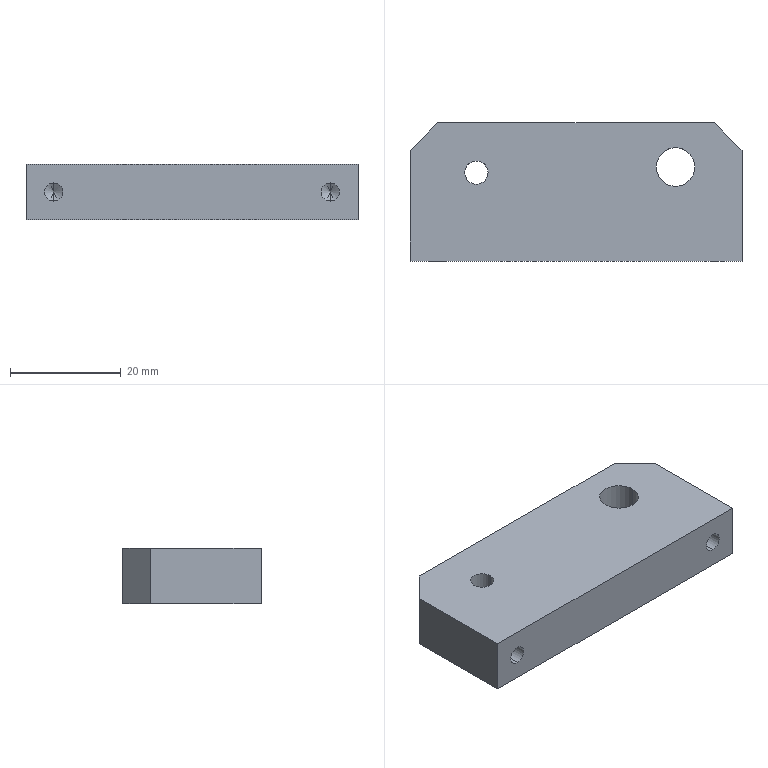Part | STEP file | 2077 Cylinder mounting plate | 1 solid | 20 faces | box 60 x 25 x 10 mm | volume 14024 mm3 | cylinder 8 | plane 8 | cone 4 | commonest cylinder face diameters 3.3 x4 4.2 x2 7 x2
STEP:
#1=CARTESIAN_POINT('',(0.,0.,0.));
#2=DIRECTION('',(0.,0.,1.));
#3=DIRECTION('',(1.,0.,0.));
#4=AXIS2_PLACEMENT_3D('',#1,#2,#3);
#5=CARTESIAN_POINT('',(-15.9,3.5,0.));
#6=VERTEX_POINT('',#5);
#7=CARTESIAN_POINT('',(-15.9,3.5,10.));
#8=VERTEX_POINT('',#7);
#9=CARTESIAN_POINT('',(-15.9,3.5,10.));
#10=DIRECTION('',(0.,0.,1.));
#11=VECTOR('',#10,1.);
#12=LINE('',#9,#11);
#13=CARTESIAN_POINT('',(-18.,3.5,10.));
#14=DIRECTION('',(0.,0.,1.));
#15=DIRECTION('',(1.,0.,0.));
#16=AXIS2_PLACEMENT_3D('',#13,#14,#15);
#17=CYLINDRICAL_SURFACE('',#16,2.1);
#18=CARTESIAN_POINT('',(6.283,0.));
#19=DIRECTION('',(0.,1.));
#20=VECTOR('',#19,1.);
#21=LINE('',#18,#20);
#22=(GEOMETRIC_REPRESENTATION_CONTEXT(2)PARAMETRIC_REPRESENTATION_CONTEXT()REPRESENTATION_CONTEXT('',''));
#23=DEFINITIONAL_REPRESENTATION('',(#21),#22);
#24=PCURVE('',#17,#23);
#25=CARTESIAN_POINT('',(-18.,3.5,10.));
#26=DIRECTION('',(0.,0.,1.));
#27=DIRECTION('',(1.,0.,0.));
#28=AXIS2_PLACEMENT_3D('',#25,#26,#27);
#29=CYLINDRICAL_SURFACE('',#28,2.1);
#30=CARTESIAN_POINT('',(0.,0.));
#31=DIRECTION('',(0.,1.));
#32=VECTOR('',#31,1.);
#33=LINE('',#30,#32);
#34=(GEOMETRIC_REPRESENTATION_CONTEXT(2)PARAMETRIC_REPRESENTATION_CONTEXT()REPRESENTATION_CONTEXT('',''));
#35=DEFINITIONAL_REPRESENTATION('',(#33),#34);
#36=PCURVE('',#29,#35);
#37=SURFACE_CURVE('',#12,(#24,#36),.PCURVE_S1.);
#38=EDGE_CURVE('',#6,#8,#37,.T.);
#39=ORIENTED_EDGE('',*,*,#38,.T.);
#40=CARTESIAN_POINT('',(-20.1,3.5,10.));
#41=VERTEX_POINT('',#40);
#42=CARTESIAN_POINT('',(-18.,3.5,10.));
#43=DIRECTION('',(0.,0.,1.));
#44=DIRECTION('',(1.,0.,0.));
#45=AXIS2_PLACEMENT_3D('',#42,#43,#44);
#46=CIRCLE('',#45,2.1);
#47=CARTESIAN_POINT('',(0.,0.));
#48=DIRECTION('',(1.,0.));
#49=VECTOR('',#48,1.);
#50=LINE('',#47,#49);
#51=(GEOMETRIC_REPRESENTATION_CONTEXT(2)PARAMETRIC_REPRESENTATION_CONTEXT()REPRESENTATION_CONTEXT('',''));
#52=DEFINITIONAL_REPRESENTATION('',(#50),#51);
#53=PCURVE('',#17,#52);
#54=CARTESIAN_POINT('',(0.,0.,10.));
#55=DIRECTION('',(0.,0.,-1.));
#56=DIRECTION('',(-1.,0.,0.));
#57=AXIS2_PLACEMENT_3D('',#54,#55,#56);
#58=PLANE('',#57);
#59=CARTESIAN_POINT('',(15.9,3.5));
#60=CARTESIAN_POINT('',(15.9,7.137));
#61=CARTESIAN_POINT('',(19.05,5.319));
#62=CARTESIAN_POINT('',(22.2,3.5));
#63=CARTESIAN_POINT('',(19.05,1.681));
#64=CARTESIAN_POINT('',(15.9,-0.1373));
#65=CARTESIAN_POINT('',(15.9,3.5));
#66=(BOUNDED_CURVE()B_SPLINE_CURVE(2,(#59,#60,#61,#62,#63,#64,#65),.UNSPECIFIED.,.T.,.F.)B_SPLINE_CURVE_WITH_KNOTS((1,2,2,2,2,1),(-2.094,0.,2.094,4.189,6.283,8.378),.UNSPECIFIED.)CURVE()GEOMETRIC_REPRESENTATION_ITEM()RATIONAL_B_SPLINE_CURVE((1.,0.5,1.,0.5,1.,0.5,1.))REPRESENTATION_ITEM(''));
#67=(GEOMETRIC_REPRESENTATION_CONTEXT(2)PARAMETRIC_REPRESENTATION_CONTEXT()REPRESENTATION_CONTEXT('',''));
#68=DEFINITIONAL_REPRESENTATION('',(#66),#67);
#69=PCURVE('',#58,#68);
#70=SURFACE_CURVE('',#46,(#53,#69),.PCURVE_S1.);
#71=EDGE_CURVE('',#41,#8,#70,.T.);
#72=ORIENTED_EDGE('',*,*,#71,.F.);
#73=CARTESIAN_POINT('',(-20.1,3.5,0.));
#74=VERTEX_POINT('',#73);
#75=CARTESIAN_POINT('',(-20.1,3.5,10.));
#76=DIRECTION('',(0.,0.,1.));
#77=VECTOR('',#76,1.);
#78=LINE('',#75,#77);
#79=CARTESIAN_POINT('',(3.142,0.));
#80=DIRECTION('',(0.,1.));
#81=VECTOR('',#80,1.);
#82=LINE('',#79,#81);
#83=(GEOMETRIC_REPRESENTATION_CONTEXT(2)PARAMETRIC_REPRESENTATION_CONTEXT()REPRESENTATION_CONTEXT('',''));
#84=DEFINITIONAL_REPRESENTATION('',(#82),#83);
#85=PCURVE('',#17,#84);
#86=CARTESIAN_POINT('',(3.142,0.));
#87=DIRECTION('',(0.,1.));
#88=VECTOR('',#87,1.);
#89=LINE('',#86,#88);
#90=(GEOMETRIC_REPRESENTATION_CONTEXT(2)PARAMETRIC_REPRESENTATION_CONTEXT()REPRESENTATION_CONTEXT('',''));
#91=DEFINITIONAL_REPRESENTATION('',(#89),#90);
#92=PCURVE('',#29,#91);
#93=SURFACE_CURVE('',#78,(#85,#92),.PCURVE_S1.);
#94=EDGE_CURVE('',#74,#41,#93,.T.);
#95=ORIENTED_EDGE('',*,*,#94,.F.);
#96=CARTESIAN_POINT('',(-18.,3.5,0.));
#97=DIRECTION('',(0.,0.,1.));
#98=DIRECTION('',(1.,0.,0.));
#99=AXIS2_PLACEMENT_3D('',#96,#97,#98);
#100=CIRCLE('',#99,2.1);
#101=CARTESIAN_POINT('',(0.,-10.));
#102=DIRECTION('',(1.,0.));
#103=VECTOR('',#102,1.);
#104=LINE('',#101,#103);
#105=(GEOMETRIC_REPRESENTATION_CONTEXT(2)PARAMETRIC_REPRESENTATION_CONTEXT()REPRESENTATION_CONTEXT('',''));
#106=DEFINITIONAL_REPRESENTATION('',(#104),#105);
#107=PCURVE('',#17,#106);
#108=CARTESIAN_POINT('',(0.,0.,0.));
#109=DIRECTION('',(0.,0.,-1.));
#110=DIRECTION('',(-1.,0.,0.));
#111=AXIS2_PLACEMENT_3D('',#108,#109,#110);
#112=PLANE('',#111);
#113=CARTESIAN_POINT('',(15.9,3.5));
#114=CARTESIAN_POINT('',(15.9,7.137));
#115=CARTESIAN_POINT('',(19.05,5.319));
#116=CARTESIAN_POINT('',(22.2,3.5));
#117=CARTESIAN_POINT('',(19.05,1.681));
#118=CARTESIAN_POINT('',(15.9,-0.1373));
#119=CARTESIAN_POINT('',(15.9,3.5));
#120=(BOUNDED_CURVE()B_SPLINE_CURVE(2,(#113,#114,#115,#116,#117,#118,#119),.UNSPECIFIED.,.T.,.F.)B_SPLINE_CURVE_WITH_KNOTS((1,2,2,2,2,1),(-2.094,0.,2.094,4.189,6.283,8.378),.UNSPECIFIED.)CURVE()GEOMETRIC_REPRESENTATION_ITEM()RATIONAL_B_SPLINE_CURVE((1.,0.5,1.,0.5,1.,0.5,1.))REPRESENTATION_ITEM(''));
#121=(GEOMETRIC_REPRESENTATION_CONTEXT(2)PARAMETRIC_REPRESENTATION_CONTEXT()REPRESENTATION_CONTEXT('',''));
#122=DEFINITIONAL_REPRESENTATION('',(#120),#121);
#123=PCURVE('',#112,#122);
#124=SURFACE_CURVE('',#100,(#107,#123),.PCURVE_S1.);
#125=EDGE_CURVE('',#74,#6,#124,.T.);
#126=ORIENTED_EDGE('',*,*,#125,.T.);
#127=EDGE_LOOP('',(#39,#72,#95,#126));
#128=FACE_BOUND('',#127,.F.);
#129=ADVANCED_FACE('',(#128),#17,.F.);
#130=CARTESIAN_POINT('',(21.5,4.5,0.));
#131=VERTEX_POINT('',#130);
#132=CARTESIAN_POINT('',(21.5,4.5,10.));
#133=VERTEX_POINT('',#132);
#134=CARTESIAN_POINT('',(21.5,4.5,10.));
#135=DIRECTION('',(0.,0.,1.));
#136=VECTOR('',#135,1.);
#137=LINE('',#134,#136);
#138=CARTESIAN_POINT('',(18.,4.5,10.));
#139=DIRECTION('',(0.,0.,1.));
#140=DIRECTION('',(1.,0.,0.));
#141=AXIS2_PLACEMENT_3D('',#138,#139,#140);
#142=CYLINDRICAL_SURFACE('',#141,3.5);
#143=CARTESIAN_POINT('',(6.283,0.));
#144=DIRECTION('',(0.,1.));
#145=VECTOR('',#144,1.);
#146=LINE('',#143,#145);
#147=(GEOMETRIC_REPRESENTATION_CONTEXT(2)PARAMETRIC_REPRESENTATION_CONTEXT()REPRESENTATION_CONTEXT('',''));
#148=DEFINITIONAL_REPRESENTATION('',(#146),#147);
#149=PCURVE('',#142,#148);
#150=CARTESIAN_POINT('',(18.,4.5,10.));
#151=DIRECTION('',(0.,0.,1.));
#152=DIRECTION('',(1.,0.,0.));
#153=AXIS2_PLACEMENT_3D('',#150,#151,#152);
#154=CYLINDRICAL_SURFACE('',#153,3.5);
#155=CARTESIAN_POINT('',(0.,0.));
#156=DIRECTION('',(0.,1.));
#157=VECTOR('',#156,1.);
#158=LINE('',#155,#157);
#159=(GEOMETRIC_REPRESENTATION_CONTEXT(2)PARAMETRIC_REPRESENTATION_CONTEXT()REPRESENTATION_CONTEXT('',''));
#160=DEFINITIONAL_REPRESENTATION('',(#158),#159);
#161=PCURVE('',#154,#160);
#162=SURFACE_CURVE('',#137,(#149,#161),.PCURVE_S1.);
#163=EDGE_CURVE('',#131,#133,#162,.T.);
#164=ORIENTED_EDGE('',*,*,#163,.T.);
#165=CARTESIAN_POINT('',(14.5,4.5,10.));
#166=VERTEX_POINT('',#165);
#167=CARTESIAN_POINT('',(18.,4.5,10.));
#168=DIRECTION('',(0.,0.,1.));
#169=DIRECTION('',(1.,0.,0.));
#170=AXIS2_PLACEMENT_3D('',#167,#168,#169);
#171=CIRCLE('',#170,3.5);
#172=CARTESIAN_POINT('',(0.,0.));
#173=DIRECTION('',(1.,0.));
#174=VECTOR('',#173,1.);
#175=LINE('',#172,#174);
#176=(GEOMETRIC_REPRESENTATION_CONTEXT(2)PARAMETRIC_REPRESENTATION_CONTEXT()REPRESENTATION_CONTEXT('',''));
#177=DEFINITIONAL_REPRESENTATION('',(#175),#176);
#178=PCURVE('',#142,#177);
#179=CARTESIAN_POINT('',(-21.5,4.5));
#180=CARTESIAN_POINT('',(-21.5,10.562));
#181=CARTESIAN_POINT('',(-16.25,7.531));
#182=CARTESIAN_POINT('',(-11.,4.5));
#183=CARTESIAN_POINT('',(-16.25,1.469));
#184=CARTESIAN_POINT('',(-21.5,-1.562));
#185=CARTESIAN_POINT('',(-21.5,4.5));
#186=(BOUNDED_CURVE()B_SPLINE_CURVE(2,(#179,#180,#181,#182,#183,#184,#185),.UNSPECIFIED.,.T.,.F.)B_SPLINE_CURVE_WITH_KNOTS((1,2,2,2,2,1),(-2.094,0.,2.094,4.189,6.283,8.378),.UNSPECIFIED.)CURVE()GEOMETRIC_REPRESENTATION_ITEM()RATIONAL_B_SPLINE_CURVE((1.,0.5,1.,0.5,1.,0.5,1.))REPRESENTATION_ITEM(''));
#187=(GEOMETRIC_REPRESENTATION_CONTEXT(2)PARAMETRIC_REPRESENTATION_CONTEXT()REPRESENTATION_CONTEXT('',''));
#188=DEFINITIONAL_REPRESENTATION('',(#186),#187);
#189=PCURVE('',#58,#188);
#190=SURFACE_CURVE('',#171,(#178,#189),.PCURVE_S1.);
#191=EDGE_CURVE('',#166,#133,#190,.T.);
#192=ORIENTED_EDGE('',*,*,#191,.F.);
#193=CARTESIAN_POINT('',(14.5,4.5,0.));
#194=VERTEX_POINT('',#193);
#195=CARTESIAN_POINT('',(14.5,4.5,10.));
#196=DIRECTION('',(0.,0.,1.));
#197=VECTOR('',#196,1.);
#198=LINE('',#195,#197);
#199=CARTESIAN_POINT('',(3.142,0.));
#200=DIRECTION('',(0.,1.));
#201=VECTOR('',#200,1.);
#202=LINE('',#199,#201);
#203=(GEOMETRIC_REPRESENTATION_CONTEXT(2)PARAMETRIC_REPRESENTATION_CONTEXT()REPRESENTATION_CONTEXT('',''));
#204=DEFINITIONAL_REPRESENTATION('',(#202),#203);
#205=PCURVE('',#142,#204);
#206=CARTESIAN_POINT('',(3.142,0.));
#207=DIRECTION('',(0.,1.));
#208=VECTOR('',#207,1.);
#209=LINE('',#206,#208);
#210=(GEOMETRIC_REPRESENTATION_CONTEXT(2)PARAMETRIC_REPRESENTATION_CONTEXT()REPRESENTATION_CONTEXT('',''));
#211=DEFINITIONAL_REPRESENTATION('',(#209),#210);
#212=PCURVE('',#154,#211);
#213=SURFACE_CURVE('',#198,(#205,#212),.PCURVE_S1.);
#214=EDGE_CURVE('',#194,#166,#213,.T.);
#215=ORIENTED_EDGE('',*,*,#214,.F.);
#216=CARTESIAN_POINT('',(18.,4.5,0.));
#217=DIRECTION('',(0.,0.,1.));
#218=DIRECTION('',(1.,0.,0.));
#219=AXIS2_PLACEMENT_3D('',#216,#217,#218);
#220=CIRCLE('',#219,3.5);
#221=CARTESIAN_POINT('',(0.,-10.));
#222=DIRECTION('',(1.,0.));
#223=VECTOR('',#222,1.);
#224=LINE('',#221,#223);
#225=(GEOMETRIC_REPRESENTATION_CONTEXT(2)PARAMETRIC_REPRESENTATION_CONTEXT()REPRESENTATION_CONTEXT('',''));
#226=DEFINITIONAL_REPRESENTATION('',(#224),#225);
#227=PCURVE('',#142,#226);
#228=CARTESIAN_POINT('',(-21.5,4.5));
#229=CARTESIAN_POINT('',(-21.5,10.562));
#230=CARTESIAN_POINT('',(-16.25,7.531));
#231=CARTESIAN_POINT('',(-11.,4.5));
#232=CARTESIAN_POINT('',(-16.25,1.469));
#233=CARTESIAN_POINT('',(-21.5,-1.562));
#234=CARTESIAN_POINT('',(-21.5,4.5));
#235=(BOUNDED_CURVE()B_SPLINE_CURVE(2,(#228,#229,#230,#231,#232,#233,#234),.UNSPECIFIED.,.T.,.F.)B_SPLINE_CURVE_WITH_KNOTS((1,2,2,2,2,1),(-2.094,0.,2.094,4.189,6.283,8.378),.UNSPECIFIED.)CURVE()GEOMETRIC_REPRESENTATION_ITEM()RATIONAL_B_SPLINE_CURVE((1.,0.5,1.,0.5,1.,0.5,1.))REPRESENTATION_ITEM(''));
#236=(GEOMETRIC_REPRESENTATION_CONTEXT(2)PARAMETRIC_REPRESENTATION_CONTEXT()REPRESENTATION_CONTEXT('',''));
#237=DEFINITIONAL_REPRESENTATION('',(#235),#236);
#238=PCURVE('',#112,#237);
#239=SURFACE_CURVE('',#220,(#227,#238),.PCURVE_S1.);
#240=EDGE_CURVE('',#194,#131,#239,.T.);
#241=ORIENTED_EDGE('',*,*,#240,.T.);
#242=EDGE_LOOP('',(#164,#192,#215,#241));
#243=FACE_BOUND('',#242,.F.);
#244=ADVANCED_FACE('',(#243),#142,.F.);
#245=CARTESIAN_POINT('',(25.,-1.,3.35));
#246=VERTEX_POINT('',#245);
#247=CARTESIAN_POINT('',(25.,-12.5,3.35));
#248=VERTEX_POINT('',#247);
#249=CARTESIAN_POINT('',(25.,-12.5,3.35));
#250=DIRECTION('',(0.,-1.,0.));
#251=VECTOR('',#250,1.);
#252=LINE('',#249,#251);
#253=CARTESIAN_POINT('',(25.,-12.5,5.));
#254=DIRECTION('',(0.,-1.,0.));
#255=DIRECTION('',(0.,0.,-1.));
#256=AXIS2_PLACEMENT_3D('',#253,#254,#255);
#257=CYLINDRICAL_SURFACE('',#256,1.65);
#258=CARTESIAN_POINT('',(6.283,0.));
#259=DIRECTION('',(0.,1.));
#260=VECTOR('',#259,1.);
#261=LINE('',#258,#260);
#262=(GEOMETRIC_REPRESENTATION_CONTEXT(2)PARAMETRIC_REPRESENTATION_CONTEXT()REPRESENTATION_CONTEXT('',''));
#263=DEFINITIONAL_REPRESENTATION('',(#261),#262);
#264=PCURVE('',#257,#263);
#265=CARTESIAN_POINT('',(25.,-12.5,5.));
#266=DIRECTION('',(0.,-1.,0.));
#267=DIRECTION('',(0.,0.,-1.));
#268=AXIS2_PLACEMENT_3D('',#265,#266,#267);
#269=CYLINDRICAL_SURFACE('',#268,1.65);
#270=CARTESIAN_POINT('',(0.,0.));
#271=DIRECTION('',(0.,1.));
#272=VECTOR('',#271,1.);
#273=LINE('',#270,#272);
#274=(GEOMETRIC_REPRESENTATION_CONTEXT(2)PARAMETRIC_REPRESENTATION_CONTEXT()REPRESENTATION_CONTEXT('',''));
#275=DEFINITIONAL_REPRESENTATION('',(#273),#274);
#276=PCURVE('',#269,#275);
#277=SURFACE_CURVE('',#252,(#264,#276),.PCURVE_S1.);
#278=EDGE_CURVE('',#246,#248,#277,.T.);
#279=ORIENTED_EDGE('',*,*,#278,.T.);
#280=CARTESIAN_POINT('',(25.,-12.5,6.65));
#281=VERTEX_POINT('',#280);
#282=CARTESIAN_POINT('',(25.,-12.5,5.));
#283=DIRECTION('',(0.,-1.,0.));
#284=DIRECTION('',(0.,0.,-1.));
#285=AXIS2_PLACEMENT_3D('',#282,#283,#284);
#286=CIRCLE('',#285,1.65);
#287=CARTESIAN_POINT('',(0.,0.));
#288=DIRECTION('',(1.,0.));
#289=VECTOR('',#288,1.);
#290=LINE('',#287,#289);
#291=(GEOMETRIC_REPRESENTATION_CONTEXT(2)PARAMETRIC_REPRESENTATION_CONTEXT()REPRESENTATION_CONTEXT('',''));
#292=DEFINITIONAL_REPRESENTATION('',(#290),#291);
#293=PCURVE('',#257,#292);
#294=CARTESIAN_POINT('',(-30.,-12.5,10.));
#295=DIRECTION('',(0.,1.,0.));
#296=DIRECTION('',(0.,0.,1.));
#297=AXIS2_PLACEMENT_3D('',#294,#295,#296);
#298=PLANE('',#297);
#299=CARTESIAN_POINT('',(-6.65,55.));
#300=CARTESIAN_POINT('',(-6.65,57.858));
#301=CARTESIAN_POINT('',(-4.175,56.429));
#302=CARTESIAN_POINT('',(-1.7,55.));
#303=CARTESIAN_POINT('',(-4.175,53.571));
#304=CARTESIAN_POINT('',(-6.65,52.142));
#305=CARTESIAN_POINT('',(-6.65,55.));
#306=(BOUNDED_CURVE()B_SPLINE_CURVE(2,(#299,#300,#301,#302,#303,#304,#305),.UNSPECIFIED.,.T.,.F.)B_SPLINE_CURVE_WITH_KNOTS((1,2,2,2,2,1),(-2.094,0.,2.094,4.189,6.283,8.378),.UNSPECIFIED.)CURVE()GEOMETRIC_REPRESENTATION_ITEM()RATIONAL_B_SPLINE_CURVE((1.,0.5,1.,0.5,1.,0.5,1.))REPRESENTATION_ITEM(''));
#307=(GEOMETRIC_REPRESENTATION_CONTEXT(2)PARAMETRIC_REPRESENTATION_CONTEXT()REPRESENTATION_CONTEXT('',''));
#308=DEFINITIONAL_REPRESENTATION('',(#306),#307);
#309=PCURVE('',#298,#308);
#310=SURFACE_CURVE('',#286,(#293,#309),.PCURVE_S1.);
#311=EDGE_CURVE('',#281,#248,#310,.T.);
#312=ORIENTED_EDGE('',*,*,#311,.F.);
#313=CARTESIAN_POINT('',(25.,-1.,6.65));
#314=VERTEX_POINT('',#313);
#315=CARTESIAN_POINT('',(25.,-12.5,6.65));
#316=DIRECTION('',(0.,-1.,0.));
#317=VECTOR('',#316,1.);
#318=LINE('',#315,#317);
#319=CARTESIAN_POINT('',(3.142,0.));
#320=DIRECTION('',(0.,1.));
#321=VECTOR('',#320,1.);
#322=LINE('',#319,#321);
#323=(GEOMETRIC_REPRESENTATION_CONTEXT(2)PARAMETRIC_REPRESENTATION_CONTEXT()REPRESENTATION_CONTEXT('',''));
#324=DEFINITIONAL_REPRESENTATION('',(#322),#323);
#325=PCURVE('',#257,#324);
#326=CARTESIAN_POINT('',(3.142,0.));
#327=DIRECTION('',(0.,1.));
#328=VECTOR('',#327,1.);
#329=LINE('',#326,#328);
#330=(GEOMETRIC_REPRESENTATION_CONTEXT(2)PARAMETRIC_REPRESENTATION_CONTEXT()REPRESENTATION_CONTEXT('',''));
#331=DEFINITIONAL_REPRESENTATION('',(#329),#330);
#332=PCURVE('',#269,#331);
#333=SURFACE_CURVE('',#318,(#325,#332),.PCURVE_S1.);
#334=EDGE_CURVE('',#314,#281,#333,.T.);
#335=ORIENTED_EDGE('',*,*,#334,.F.);
#336=CARTESIAN_POINT('',(25.,-1.,5.));
#337=DIRECTION('',(0.,-1.,0.));
#338=DIRECTION('',(0.,0.,-1.));
#339=AXIS2_PLACEMENT_3D('',#336,#337,#338);
#340=CIRCLE('',#339,1.65);
#341=CARTESIAN_POINT('',(0.,-11.5));
#342=DIRECTION('',(1.,0.));
#343=VECTOR('',#342,1.);
#344=LINE('',#341,#343);
#345=(GEOMETRIC_REPRESENTATION_CONTEXT(2)PARAMETRIC_REPRESENTATION_CONTEXT()REPRESENTATION_CONTEXT('',''));
#346=DEFINITIONAL_REPRESENTATION('',(#344),#345);
#347=PCURVE('',#257,#346);
#348=CARTESIAN_POINT('',(25.,-1.,5.));
#349=DIRECTION('',(0.,-1.,0.));
#350=DIRECTION('',(0.,0.,-1.));
#351=AXIS2_PLACEMENT_3D('',#348,#349,#350);
#352=CONICAL_SURFACE('',#351,1.65,1.03);
#353=CARTESIAN_POINT('',(0.,0.));
#354=DIRECTION('',(1.,0.));
#355=VECTOR('',#354,1.);
#356=LINE('',#353,#355);
#357=(GEOMETRIC_REPRESENTATION_CONTEXT(2)PARAMETRIC_REPRESENTATION_CONTEXT()REPRESENTATION_CONTEXT('',''));
#358=DEFINITIONAL_REPRESENTATION('',(#356),#357);
#359=PCURVE('',#352,#358);
#360=SURFACE_CURVE('',#340,(#347,#359),.PCURVE_S1.);
#361=EDGE_CURVE('',#314,#246,#360,.T.);
#362=ORIENTED_EDGE('',*,*,#361,.T.);
#363=EDGE_LOOP('',(#279,#312,#335,#362));
#364=FACE_BOUND('',#363,.F.);
#365=ADVANCED_FACE('',(#364),#257,.F.);
#366=ORIENTED_EDGE('',*,*,#361,.F.);
#367=CARTESIAN_POINT('',(25.,-0.00858,5.));
#368=VERTEX_POINT('',#367);
#369=CARTESIAN_POINT('',(25.,-1.,6.65));
#370=DIRECTION('',(0.,-0.515,0.8572));
#371=VECTOR('',#370,1.);
#372=LINE('',#369,#371);
#373=CARTESIAN_POINT('',(3.142,0.));
#374=DIRECTION('',(0.,1.));
#375=VECTOR('',#374,1.);
#376=LINE('',#373,#375);
#377=(GEOMETRIC_REPRESENTATION_CONTEXT(2)PARAMETRIC_REPRESENTATION_CONTEXT()REPRESENTATION_CONTEXT('',''));
#378=DEFINITIONAL_REPRESENTATION('',(#376),#377);
#379=PCURVE('',#352,#378);
#380=CARTESIAN_POINT('',(25.,-1.,5.));
#381=DIRECTION('',(0.,-1.,0.));
#382=DIRECTION('',(0.,0.,-1.));
#383=AXIS2_PLACEMENT_3D('',#380,#381,#382);
#384=CONICAL_SURFACE('',#383,1.65,1.03);
#385=CARTESIAN_POINT('',(3.142,0.));
#386=DIRECTION('',(0.,1.));
#387=VECTOR('',#386,1.);
#388=LINE('',#385,#387);
#389=(GEOMETRIC_REPRESENTATION_CONTEXT(2)PARAMETRIC_REPRESENTATION_CONTEXT()REPRESENTATION_CONTEXT('',''));
#390=DEFINITIONAL_REPRESENTATION('',(#388),#389);
#391=PCURVE('',#384,#390);
#392=SURFACE_CURVE('',#372,(#379,#391),.PCURVE_S1.);
#393=EDGE_CURVE('',#368,#314,#392,.T.);
#394=ORIENTED_EDGE('',*,*,#393,.F.);
#395=CARTESIAN_POINT('',(25.,-1.,3.35));
#396=DIRECTION('',(0.,-0.515,-0.8572));
#397=VECTOR('',#396,1.);
#398=LINE('',#395,#397);
#399=CARTESIAN_POINT('',(6.283,0.));
#400=DIRECTION('',(0.,1.));
#401=VECTOR('',#400,1.);
#402=LINE('',#399,#401);
#403=(GEOMETRIC_REPRESENTATION_CONTEXT(2)PARAMETRIC_REPRESENTATION_CONTEXT()REPRESENTATION_CONTEXT('',''));
#404=DEFINITIONAL_REPRESENTATION('',(#402),#403);
#405=PCURVE('',#352,#404);
#406=CARTESIAN_POINT('',(0.,0.));
#407=DIRECTION('',(0.,1.));
#408=VECTOR('',#407,1.);
#409=LINE('',#406,#408);
#410=(GEOMETRIC_REPRESENTATION_CONTEXT(2)PARAMETRIC_REPRESENTATION_CONTEXT()REPRESENTATION_CONTEXT('',''));
#411=DEFINITIONAL_REPRESENTATION('',(#409),#410);
#412=PCURVE('',#384,#411);
#413=SURFACE_CURVE('',#398,(#405,#412),.PCURVE_S1.);
#414=EDGE_CURVE('',#368,#246,#413,.T.);
#415=ORIENTED_EDGE('',*,*,#414,.T.);
#416=EDGE_LOOP('',(#366,#394,#415));
#417=FACE_BOUND('',#416,.F.);
#418=ADVANCED_FACE('',(#417),#352,.F.);
#419=CARTESIAN_POINT('',(-25.,-1.,3.35));
#420=VERTEX_POINT('',#419);
#421=CARTESIAN_POINT('',(-25.,-12.5,3.35));
#422=VERTEX_POINT('',#421);
#423=CARTESIAN_POINT('',(-25.,-12.5,3.35));
#424=DIRECTION('',(0.,-1.,0.));
#425=VECTOR('',#424,1.);
#426=LINE('',#423,#425);
#427=CARTESIAN_POINT('',(-25.,-12.5,5.));
#428=DIRECTION('',(0.,-1.,0.));
#429=DIRECTION('',(0.,0.,-1.));
#430=AXIS2_PLACEMENT_3D('',#427,#428,#429);
#431=CYLINDRICAL_SURFACE('',#430,1.65);
#432=CARTESIAN_POINT('',(6.283,0.));
#433=DIRECTION('',(0.,1.));
#434=VECTOR('',#433,1.);
#435=LINE('',#432,#434);
#436=(GEOMETRIC_REPRESENTATION_CONTEXT(2)PARAMETRIC_REPRESENTATION_CONTEXT()REPRESENTATION_CONTEXT('',''));
#437=DEFINITIONAL_REPRESENTATION('',(#435),#436);
#438=PCURVE('',#431,#437);
#439=CARTESIAN_POINT('',(-25.,-12.5,5.));
#440=DIRECTION('',(0.,-1.,0.));
#441=DIRECTION('',(0.,0.,-1.));
#442=AXIS2_PLACEMENT_3D('',#439,#440,#441);
#443=CYLINDRICAL_SURFACE('',#442,1.65);
#444=CARTESIAN_POINT('',(0.,0.));
#445=DIRECTION('',(0.,1.));
#446=VECTOR('',#445,1.);
#447=LINE('',#444,#446);
#448=(GEOMETRIC_REPRESENTATION_CONTEXT(2)PARAMETRIC_REPRESENTATION_CONTEXT()REPRESENTATION_CONTEXT('',''));
#449=DEFINITIONAL_REPRESENTATION('',(#447),#448);
#450=PCURVE('',#443,#449);
#451=SURFACE_CURVE('',#426,(#438,#450),.PCURVE_S1.);
#452=EDGE_CURVE('',#420,#422,#451,.T.);
#453=ORIENTED_EDGE('',*,*,#452,.T.);
#454=CARTESIAN_POINT('',(-25.,-12.5,6.65));
#455=VERTEX_POINT('',#454);
#456=CARTESIAN_POINT('',(-25.,-12.5,5.));
#457=DIRECTION('',(0.,-1.,0.));
#458=DIRECTION('',(0.,0.,-1.));
#459=AXIS2_PLACEMENT_3D('',#456,#457,#458);
#460=CIRCLE('',#459,1.65);
#461=CARTESIAN_POINT('',(0.,0.));
#462=DIRECTION('',(1.,0.));
#463=VECTOR('',#462,1.);
#464=LINE('',#461,#463);
#465=(GEOMETRIC_REPRESENTATION_CONTEXT(2)PARAMETRIC_REPRESENTATION_CONTEXT()REPRESENTATION_CONTEXT('',''));
#466=DEFINITIONAL_REPRESENTATION('',(#464),#465);
#467=PCURVE('',#431,#466);
#468=CARTESIAN_POINT('',(-6.65,5.));
#469=CARTESIAN_POINT('',(-6.65,7.858));
#470=CARTESIAN_POINT('',(-4.175,6.429));
#471=CARTESIAN_POINT('',(-1.7,5.));
#472=CARTESIAN_POINT('',(-4.175,3.571));
#473=CARTESIAN_POINT('',(-6.65,2.142));
#474=CARTESIAN_POINT('',(-6.65,5.));
#475=(BOUNDED_CURVE()B_SPLINE_CURVE(2,(#468,#469,#470,#471,#472,#473,#474),.UNSPECIFIED.,.T.,.F.)B_SPLINE_CURVE_WITH_KNOTS((1,2,2,2,2,1),(-2.094,0.,2.094,4.189,6.283,8.378),.UNSPECIFIED.)CURVE()GEOMETRIC_REPRESENTATION_ITEM()RATIONAL_B_SPLINE_CURVE((1.,0.5,1.,0.5,1.,0.5,1.))REPRESENTATION_ITEM(''));
#476=(GEOMETRIC_REPRESENTATION_CONTEXT(2)PARAMETRIC_REPRESENTATION_CONTEXT()REPRESENTATION_CONTEXT('',''));
#477=DEFINITIONAL_REPRESENTATION('',(#475),#476);
#478=PCURVE('',#298,#477);
#479=SURFACE_CURVE('',#460,(#467,#478),.PCURVE_S1.);
#480=EDGE_CURVE('',#455,#422,#479,.T.);
#481=ORIENTED_EDGE('',*,*,#480,.F.);
#482=CARTESIAN_POINT('',(-25.,-1.,6.65));
#483=VERTEX_POINT('',#482);
#484=CARTESIAN_POINT('',(-25.,-12.5,6.65));
#485=DIRECTION('',(0.,-1.,0.));
#486=VECTOR('',#485,1.);
#487=LINE('',#484,#486);
#488=CARTESIAN_POINT('',(3.142,0.));
#489=DIRECTION('',(0.,1.));
#490=VECTOR('',#489,1.);
#491=LINE('',#488,#490);
#492=(GEOMETRIC_REPRESENTATION_CONTEXT(2)PARAMETRIC_REPRESENTATION_CONTEXT()REPRESENTATION_CONTEXT('',''));
#493=DEFINITIONAL_REPRESENTATION('',(#491),#492);
#494=PCURVE('',#431,#493);
#495=CARTESIAN_POINT('',(3.142,0.));
#496=DIRECTION('',(0.,1.));
#497=VECTOR('',#496,1.);
#498=LINE('',#495,#497);
#499=(GEOMETRIC_REPRESENTATION_CONTEXT(2)PARAMETRIC_REPRESENTATION_CONTEXT()REPRESENTATION_CONTEXT('',''));
#500=DEFINITIONAL_REPRESENTATION('',(#498),#499);
#501=PCURVE('',#443,#500);
#502=SURFACE_CURVE('',#487,(#494,#501),.PCURVE_S1.);
#503=EDGE_CURVE('',#483,#455,#502,.T.);
#504=ORIENTED_EDGE('',*,*,#503,.F.);
#505=CARTESIAN_POINT('',(-25.,-1.,5.));
#506=DIRECTION('',(0.,-1.,0.));
#507=DIRECTION('',(0.,0.,-1.));
#508=AXIS2_PLACEMENT_3D('',#505,#506,#507);
#509=CIRCLE('',#508,1.65);
#510=CARTESIAN_POINT('',(0.,-11.5));
#511=DIRECTION('',(1.,0.));
#512=VECTOR('',#511,1.);
#513=LINE('',#510,#512);
#514=(GEOMETRIC_REPRESENTATION_CONTEXT(2)PARAMETRIC_REPRESENTATION_CONTEXT()REPRESENTATION_CONTEXT('',''));
#515=DEFINITIONAL_REPRESENTATION('',(#513),#514);
#516=PCURVE('',#431,#515);
#517=CARTESIAN_POINT('',(-25.,-1.,5.));
#518=DIRECTION('',(0.,-1.,0.));
#519=DIRECTION('',(0.,0.,-1.));
#520=AXIS2_PLACEMENT_3D('',#517,#518,#519);
#521=CONICAL_SURFACE('',#520,1.65,1.03);
#522=CARTESIAN_POINT('',(0.,0.));
#523=DIRECTION('',(1.,0.));
#524=VECTOR('',#523,1.);
#525=LINE('',#522,#524);
#526=(GEOMETRIC_REPRESENTATION_CONTEXT(2)PARAMETRIC_REPRESENTATION_CONTEXT()REPRESENTATION_CONTEXT('',''));
#527=DEFINITIONAL_REPRESENTATION('',(#525),#526);
#528=PCURVE('',#521,#527);
#529=SURFACE_CURVE('',#509,(#516,#528),.PCURVE_S1.);
#530=EDGE_CURVE('',#483,#420,#529,.T.);
#531=ORIENTED_EDGE('',*,*,#530,.T.);
#532=EDGE_LOOP('',(#453,#481,#504,#531));
#533=FACE_BOUND('',#532,.F.);
#534=ADVANCED_FACE('',(#533),#431,.F.);
#535=ORIENTED_EDGE('',*,*,#530,.F.);
#536=CARTESIAN_POINT('',(-25.,-0.00858,5.));
#537=VERTEX_POINT('',#536);
#538=CARTESIAN_POINT('',(-25.,-1.,6.65));
#539=DIRECTION('',(0.,-0.515,0.8572));
#540=VECTOR('',#539,1.);
#541=LINE('',#538,#540);
#542=CARTESIAN_POINT('',(3.142,0.));
#543=DIRECTION('',(0.,1.));
#544=VECTOR('',#543,1.);
#545=LINE('',#542,#544);
#546=(GEOMETRIC_REPRESENTATION_CONTEXT(2)PARAMETRIC_REPRESENTATION_CONTEXT()REPRESENTATION_CONTEXT('',''));
#547=DEFINITIONAL_REPRESENTATION('',(#545),#546);
#548=PCURVE('',#521,#547);
#549=CARTESIAN_POINT('',(-25.,-1.,5.));
#550=DIRECTION('',(0.,-1.,0.));
#551=DIRECTION('',(0.,0.,-1.));
#552=AXIS2_PLACEMENT_3D('',#549,#550,#551);
#553=CONICAL_SURFACE('',#552,1.65,1.03);
#554=CARTESIAN_POINT('',(3.142,0.));
#555=DIRECTION('',(0.,1.));
#556=VECTOR('',#555,1.);
#557=LINE('',#554,#556);
#558=(GEOMETRIC_REPRESENTATION_CONTEXT(2)PARAMETRIC_REPRESENTATION_CONTEXT()REPRESENTATION_CONTEXT('',''));
#559=DEFINITIONAL_REPRESENTATION('',(#557),#558);
#560=PCURVE('',#553,#559);
#561=SURFACE_CURVE('',#541,(#548,#560),.PCURVE_S1.);
#562=EDGE_CURVE('',#537,#483,#561,.T.);
#563=ORIENTED_EDGE('',*,*,#562,.F.);
#564=CARTESIAN_POINT('',(-25.,-1.,3.35));
#565=DIRECTION('',(0.,-0.515,-0.8572));
#566=VECTOR('',#565,1.);
#567=LINE('',#564,#566);
#568=CARTESIAN_POINT('',(6.283,0.));
#569=DIRECTION('',(0.,1.));
#570=VECTOR('',#569,1.);
#571=LINE('',#568,#570);
#572=(GEOMETRIC_REPRESENTATION_CONTEXT(2)PARAMETRIC_REPRESENTATION_CONTEXT()REPRESENTATION_CONTEXT('',''));
#573=DEFINITIONAL_REPRESENTATION('',(#571),#572);
#574=PCURVE('',#521,#573);
#575=CARTESIAN_POINT('',(0.,0.));
#576=DIRECTION('',(0.,1.));
#577=VECTOR('',#576,1.);
#578=LINE('',#575,#577);
#579=(GEOMETRIC_REPRESENTATION_CONTEXT(2)PARAMETRIC_REPRESENTATION_CONTEXT()REPRESENTATION_CONTEXT('',''));
#580=DEFINITIONAL_REPRESENTATION('',(#578),#579);
#581=PCURVE('',#553,#580);
#582=SURFACE_CURVE('',#567,(#574,#581),.PCURVE_S1.);
#583=EDGE_CURVE('',#537,#420,#582,.T.);
#584=ORIENTED_EDGE('',*,*,#583,.T.);
#585=EDGE_LOOP('',(#535,#563,#584));
#586=FACE_BOUND('',#585,.F.);
#587=ADVANCED_FACE('',(#586),#521,.F.);
#588=CARTESIAN_POINT('',(30.,-12.5,0.));
#589=VERTEX_POINT('',#588);
#590=CARTESIAN_POINT('',(30.,7.5,0.));
#591=VERTEX_POINT('',#590);
#592=CARTESIAN_POINT('',(30.,-12.5,0.));
#593=DIRECTION('',(0.,1.,0.));
#594=VECTOR('',#593,1.);
#595=LINE('',#592,#594);
#596=CARTESIAN_POINT('',(30.,-12.5,10.));
#597=DIRECTION('',(-1.,0.,0.));
#598=DIRECTION('',(0.,0.,1.));
#599=AXIS2_PLACEMENT_3D('',#596,#597,#598);
#600=PLANE('',#599);
#601=CARTESIAN_POINT('',(-10.,0.));
#602=DIRECTION('',(0.,1.));
#603=VECTOR('',#602,1.);
#604=LINE('',#601,#603);
#605=(GEOMETRIC_REPRESENTATION_CONTEXT(2)PARAMETRIC_REPRESENTATION_CONTEXT()REPRESENTATION_CONTEXT('',''));
#606=DEFINITIONAL_REPRESENTATION('',(#604),#605);
#607=PCURVE('',#600,#606);
#608=CARTESIAN_POINT('',(-30.,-12.5));
#609=DIRECTION('',(0.,1.));
#610=VECTOR('',#609,1.);
#611=LINE('',#608,#610);
#612=(GEOMETRIC_REPRESENTATION_CONTEXT(2)PARAMETRIC_REPRESENTATION_CONTEXT()REPRESENTATION_CONTEXT('',''));
#613=DEFINITIONAL_REPRESENTATION('',(#611),#612);
#614=PCURVE('',#112,#613);
#615=SURFACE_CURVE('',#595,(#607,#614),.PCURVE_S1.);
#616=EDGE_CURVE('',#589,#591,#615,.T.);
#617=ORIENTED_EDGE('',*,*,#616,.T.);
#618=CARTESIAN_POINT('',(30.,7.5,10.));
#619=VERTEX_POINT('',#618);
#620=CARTESIAN_POINT('',(30.,7.5,10.));
#621=DIRECTION('',(0.,0.,1.));
#622=VECTOR('',#621,1.);
#623=LINE('',#620,#622);
#624=CARTESIAN_POINT('',(0.,20.));
#625=DIRECTION('',(1.,0.));
#626=VECTOR('',#625,1.);
#627=LINE('',#624,#626);
#628=(GEOMETRIC_REPRESENTATION_CONTEXT(2)PARAMETRIC_REPRESENTATION_CONTEXT()REPRESENTATION_CONTEXT('',''));
#629=DEFINITIONAL_REPRESENTATION('',(#627),#628);
#630=PCURVE('',#600,#629);
#631=CARTESIAN_POINT('',(25.,12.5,10.));
#632=DIRECTION('',(-0.7071,-0.7071,0.));
#633=DIRECTION('',(0.,0.,-1.));
#634=AXIS2_PLACEMENT_3D('',#631,#632,#633);
#635=PLANE('',#634);
#636=CARTESIAN_POINT('',(0.,7.071));
#637=DIRECTION('',(-1.,0.));
#638=VECTOR('',#637,1.);
#639=LINE('',#636,#638);
#640=(GEOMETRIC_REPRESENTATION_CONTEXT(2)PARAMETRIC_REPRESENTATION_CONTEXT()REPRESENTATION_CONTEXT('',''));
#641=DEFINITIONAL_REPRESENTATION('',(#639),#640);
#642=PCURVE('',#635,#641);
#643=SURFACE_CURVE('',#623,(#630,#642),.PCURVE_S1.);
#644=EDGE_CURVE('',#591,#619,#643,.T.);
#645=ORIENTED_EDGE('',*,*,#644,.T.);
#646=CARTESIAN_POINT('',(30.,-12.5,10.));
#647=VERTEX_POINT('',#646);
#648=CARTESIAN_POINT('',(30.,-12.5,10.));
#649=DIRECTION('',(0.,1.,0.));
#650=VECTOR('',#649,1.);
#651=LINE('',#648,#650);
#652=CARTESIAN_POINT('',(0.,0.));
#653=DIRECTION('',(0.,1.));
#654=VECTOR('',#653,1.);
#655=LINE('',#652,#654);
#656=(GEOMETRIC_REPRESENTATION_CONTEXT(2)PARAMETRIC_REPRESENTATION_CONTEXT()REPRESENTATION_CONTEXT('',''));
#657=DEFINITIONAL_REPRESENTATION('',(#655),#656);
#658=PCURVE('',#600,#657);
#659=CARTESIAN_POINT('',(-30.,-12.5));
#660=DIRECTION('',(0.,1.));
#661=VECTOR('',#660,1.);
#662=LINE('',#659,#661);
#663=(GEOMETRIC_REPRESENTATION_CONTEXT(2)PARAMETRIC_REPRESENTATION_CONTEXT()REPRESENTATION_CONTEXT('',''));
#664=DEFINITIONAL_REPRESENTATION('',(#662),#663);
#665=PCURVE('',#58,#664);
#666=SURFACE_CURVE('',#651,(#658,#665),.PCURVE_S1.);
#667=EDGE_CURVE('',#647,#619,#666,.T.);
#668=ORIENTED_EDGE('',*,*,#667,.F.);
#669=CARTESIAN_POINT('',(30.,-12.5,10.));
#670=DIRECTION('',(0.,0.,-1.));
#671=VECTOR('',#670,1.);
#672=LINE('',#669,#671);
#673=CARTESIAN_POINT('',(0.,0.));
#674=DIRECTION('',(-1.,0.));
#675=VECTOR('',#674,1.);
#676=LINE('',#673,#675);
#677=(GEOMETRIC_REPRESENTATION_CONTEXT(2)PARAMETRIC_REPRESENTATION_CONTEXT()REPRESENTATION_CONTEXT('',''));
#678=DEFINITIONAL_REPRESENTATION('',(#676),#677);
#679=PCURVE('',#600,#678);
#680=CARTESIAN_POINT('',(0.,60.));
#681=DIRECTION('',(-1.,0.));
#682=VECTOR('',#681,1.);
#683=LINE('',#680,#682);
#684=(GEOMETRIC_REPRESENTATION_CONTEXT(2)PARAMETRIC_REPRESENTATION_CONTEXT()REPRESENTATION_CONTEXT('',''));
#685=DEFINITIONAL_REPRESENTATION('',(#683),#684);
#686=PCURVE('',#298,#685);
#687=SURFACE_CURVE('',#672,(#679,#686),.PCURVE_S1.);
#688=EDGE_CURVE('',#647,#589,#687,.T.);
#689=ORIENTED_EDGE('',*,*,#688,.T.);
#690=EDGE_LOOP('',(#617,#645,#668,#689));
#691=FACE_BOUND('',#690,.T.);
#692=ADVANCED_FACE('',(#691),#600,.F.);
#693=CARTESIAN_POINT('',(25.,12.5,0.));
#694=VERTEX_POINT('',#693);
#695=CARTESIAN_POINT('',(-25.,12.5,0.));
#696=VERTEX_POINT('',#695);
#697=CARTESIAN_POINT('',(-30.,12.5,0.));
#698=DIRECTION('',(-1.,0.,0.));
#699=VECTOR('',#698,1.);
#700=LINE('',#697,#699);
#701=CARTESIAN_POINT('',(-30.,12.5,10.));
#702=DIRECTION('',(0.,-1.,0.));
#703=DIRECTION('',(0.,0.,-1.));
#704=AXIS2_PLACEMENT_3D('',#701,#702,#703);
#705=PLANE('',#704);
#706=CARTESIAN_POINT('',(10.,0.));
#707=DIRECTION('',(0.,-1.));
#708=VECTOR('',#707,1.);
#709=LINE('',#706,#708);
#710=(GEOMETRIC_REPRESENTATION_CONTEXT(2)PARAMETRIC_REPRESENTATION_CONTEXT()REPRESENTATION_CONTEXT('',''));
#711=DEFINITIONAL_REPRESENTATION('',(#709),#710);
#712=PCURVE('',#705,#711);
#713=CARTESIAN_POINT('',(30.,12.5));
#714=DIRECTION('',(1.,0.));
#715=VECTOR('',#714,1.);
#716=LINE('',#713,#715);
#717=(GEOMETRIC_REPRESENTATION_CONTEXT(2)PARAMETRIC_REPRESENTATION_CONTEXT()REPRESENTATION_CONTEXT('',''));
#718=DEFINITIONAL_REPRESENTATION('',(#716),#717);
#719=PCURVE('',#112,#718);
#720=SURFACE_CURVE('',#700,(#712,#719),.PCURVE_S1.);
#721=EDGE_CURVE('',#694,#696,#720,.T.);
#722=ORIENTED_EDGE('',*,*,#721,.T.);
#723=CARTESIAN_POINT('',(-25.,12.5,10.));
#724=VERTEX_POINT('',#723);
#725=CARTESIAN_POINT('',(-25.,12.5,10.));
#726=DIRECTION('',(0.,0.,1.));
#727=VECTOR('',#726,1.);
#728=LINE('',#725,#727);
#729=CARTESIAN_POINT('',(0.,5.));
#730=DIRECTION('',(-1.,0.));
#731=VECTOR('',#730,1.);
#732=LINE('',#729,#731);
#733=(GEOMETRIC_REPRESENTATION_CONTEXT(2)PARAMETRIC_REPRESENTATION_CONTEXT()REPRESENTATION_CONTEXT('',''));
#734=DEFINITIONAL_REPRESENTATION('',(#732),#733);
#735=PCURVE('',#705,#734);
#736=CARTESIAN_POINT('',(-30.,7.5,10.));
#737=DIRECTION('',(0.7071,-0.7071,0.));
#738=DIRECTION('',(0.,0.,-1.));
#739=AXIS2_PLACEMENT_3D('',#736,#737,#738);
#740=PLANE('',#739);
#741=CARTESIAN_POINT('',(0.,7.071));
#742=DIRECTION('',(-1.,0.));
#743=VECTOR('',#742,1.);
#744=LINE('',#741,#743);
#745=(GEOMETRIC_REPRESENTATION_CONTEXT(2)PARAMETRIC_REPRESENTATION_CONTEXT()REPRESENTATION_CONTEXT('',''));
#746=DEFINITIONAL_REPRESENTATION('',(#744),#745);
#747=PCURVE('',#740,#746);
#748=SURFACE_CURVE('',#728,(#735,#747),.PCURVE_S1.);
#749=EDGE_CURVE('',#696,#724,#748,.T.);
#750=ORIENTED_EDGE('',*,*,#749,.T.);
#751=CARTESIAN_POINT('',(25.,12.5,10.));
#752=VERTEX_POINT('',#751);
#753=CARTESIAN_POINT('',(-30.,12.5,10.));
#754=DIRECTION('',(-1.,0.,0.));
#755=VECTOR('',#754,1.);
#756=LINE('',#753,#755);
#757=CARTESIAN_POINT('',(0.,0.));
#758=DIRECTION('',(0.,-1.));
#759=VECTOR('',#758,1.);
#760=LINE('',#757,#759);
#761=(GEOMETRIC_REPRESENTATION_CONTEXT(2)PARAMETRIC_REPRESENTATION_CONTEXT()REPRESENTATION_CONTEXT('',''));
#762=DEFINITIONAL_REPRESENTATION('',(#760),#761);
#763=PCURVE('',#705,#762);
#764=CARTESIAN_POINT('',(30.,12.5));
#765=DIRECTION('',(1.,0.));
#766=VECTOR('',#765,1.);
#767=LINE('',#764,#766);
#768=(GEOMETRIC_REPRESENTATION_CONTEXT(2)PARAMETRIC_REPRESENTATION_CONTEXT()REPRESENTATION_CONTEXT('',''));
#769=DEFINITIONAL_REPRESENTATION('',(#767),#768);
#770=PCURVE('',#58,#769);
#771=SURFACE_CURVE('',#756,(#763,#770),.PCURVE_S1.);
#772=EDGE_CURVE('',#752,#724,#771,.T.);
#773=ORIENTED_EDGE('',*,*,#772,.F.);
#774=CARTESIAN_POINT('',(25.,12.5,10.));
#775=DIRECTION('',(0.,0.,-1.));
#776=VECTOR('',#775,1.);
#777=LINE('',#774,#776);
#778=CARTESIAN_POINT('',(0.,55.));
#779=DIRECTION('',(1.,0.));
#780=VECTOR('',#779,1.);
#781=LINE('',#778,#780);
#782=(GEOMETRIC_REPRESENTATION_CONTEXT(2)PARAMETRIC_REPRESENTATION_CONTEXT()REPRESENTATION_CONTEXT('',''));
#783=DEFINITIONAL_REPRESENTATION('',(#781),#782);
#784=PCURVE('',#705,#783);
#785=CARTESIAN_POINT('',(0.,0.));
#786=DIRECTION('',(1.,0.));
#787=VECTOR('',#786,1.);
#788=LINE('',#785,#787);
#789=(GEOMETRIC_REPRESENTATION_CONTEXT(2)PARAMETRIC_REPRESENTATION_CONTEXT()REPRESENTATION_CONTEXT('',''));
#790=DEFINITIONAL_REPRESENTATION('',(#788),#789);
#791=PCURVE('',#635,#790);
#792=SURFACE_CURVE('',#777,(#784,#791),.PCURVE_S1.);
#793=EDGE_CURVE('',#752,#694,#792,.T.);
#794=ORIENTED_EDGE('',*,*,#793,.T.);
#795=EDGE_LOOP('',(#722,#750,#773,#794));
#796=FACE_BOUND('',#795,.T.);
#797=ADVANCED_FACE('',(#796),#705,.F.);
#798=CARTESIAN_POINT('',(-30.,7.5,10.));
#799=VERTEX_POINT('',#798);
#800=CARTESIAN_POINT('',(-30.,-12.5,10.));
#801=VERTEX_POINT('',#800);
#802=CARTESIAN_POINT('',(-30.,-12.5,10.));
#803=DIRECTION('',(0.,-1.,0.));
#804=VECTOR('',#803,1.);
#805=LINE('',#802,#804);
#806=CARTESIAN_POINT('',(-30.,-12.5,10.));
#807=DIRECTION('',(1.,0.,0.));
#808=DIRECTION('',(0.,0.,-1.));
#809=AXIS2_PLACEMENT_3D('',#806,#807,#808);
#810=PLANE('',#809);
#811=CARTESIAN_POINT('',(0.,0.));
#812=DIRECTION('',(0.,-1.));
#813=VECTOR('',#812,1.);
#814=LINE('',#811,#813);
#815=(GEOMETRIC_REPRESENTATION_CONTEXT(2)PARAMETRIC_REPRESENTATION_CONTEXT()REPRESENTATION_CONTEXT('',''));
#816=DEFINITIONAL_REPRESENTATION('',(#814),#815);
#817=PCURVE('',#810,#816);
#818=CARTESIAN_POINT('',(30.,-12.5));
#819=DIRECTION('',(0.,-1.));
#820=VECTOR('',#819,1.);
#821=LINE('',#818,#820);
#822=(GEOMETRIC_REPRESENTATION_CONTEXT(2)PARAMETRIC_REPRESENTATION_CONTEXT()REPRESENTATION_CONTEXT('',''));
#823=DEFINITIONAL_REPRESENTATION('',(#821),#822);
#824=PCURVE('',#58,#823);
#825=SURFACE_CURVE('',#805,(#817,#824),.PCURVE_S1.);
#826=EDGE_CURVE('',#799,#801,#825,.T.);
#827=ORIENTED_EDGE('',*,*,#826,.F.);
#828=CARTESIAN_POINT('',(-30.,7.5,0.));
#829=VERTEX_POINT('',#828);
#830=CARTESIAN_POINT('',(-30.,7.5,10.));
#831=DIRECTION('',(0.,0.,-1.));
#832=VECTOR('',#831,1.);
#833=LINE('',#830,#832);
#834=CARTESIAN_POINT('',(0.,20.));
#835=DIRECTION('',(1.,0.));
#836=VECTOR('',#835,1.);
#837=LINE('',#834,#836);
#838=(GEOMETRIC_REPRESENTATION_CONTEXT(2)PARAMETRIC_REPRESENTATION_CONTEXT()REPRESENTATION_CONTEXT('',''));
#839=DEFINITIONAL_REPRESENTATION('',(#837),#838);
#840=PCURVE('',#810,#839);
#841=CARTESIAN_POINT('',(0.,0.));
#842=DIRECTION('',(1.,0.));
#843=VECTOR('',#842,1.);
#844=LINE('',#841,#843);
#845=(GEOMETRIC_REPRESENTATION_CONTEXT(2)PARAMETRIC_REPRESENTATION_CONTEXT()REPRESENTATION_CONTEXT('',''));
#846=DEFINITIONAL_REPRESENTATION('',(#844),#845);
#847=PCURVE('',#740,#846);
#848=SURFACE_CURVE('',#833,(#840,#847),.PCURVE_S1.);
#849=EDGE_CURVE('',#799,#829,#848,.T.);
#850=ORIENTED_EDGE('',*,*,#849,.T.);
#851=CARTESIAN_POINT('',(-30.,-12.5,0.));
#852=VERTEX_POINT('',#851);
#853=CARTESIAN_POINT('',(-30.,-12.5,0.));
#854=DIRECTION('',(0.,-1.,0.));
#855=VECTOR('',#854,1.);
#856=LINE('',#853,#855);
#857=CARTESIAN_POINT('',(10.,0.));
#858=DIRECTION('',(0.,-1.));
#859=VECTOR('',#858,1.);
#860=LINE('',#857,#859);
#861=(GEOMETRIC_REPRESENTATION_CONTEXT(2)PARAMETRIC_REPRESENTATION_CONTEXT()REPRESENTATION_CONTEXT('',''));
#862=DEFINITIONAL_REPRESENTATION('',(#860),#861);
#863=PCURVE('',#810,#862);
#864=CARTESIAN_POINT('',(30.,-12.5));
#865=DIRECTION('',(0.,-1.));
#866=VECTOR('',#865,1.);
#867=LINE('',#864,#866);
#868=(GEOMETRIC_REPRESENTATION_CONTEXT(2)PARAMETRIC_REPRESENTATION_CONTEXT()REPRESENTATION_CONTEXT('',''));
#869=DEFINITIONAL_REPRESENTATION('',(#867),#868);
#870=PCURVE('',#112,#869);
#871=SURFACE_CURVE('',#856,(#863,#870),.PCURVE_S1.);
#872=EDGE_CURVE('',#829,#852,#871,.T.);
#873=ORIENTED_EDGE('',*,*,#872,.T.);
#874=CARTESIAN_POINT('',(-30.,-12.5,10.));
#875=DIRECTION('',(0.,0.,-1.));
#876=VECTOR('',#875,1.);
#877=LINE('',#874,#876);
#878=CARTESIAN_POINT('',(0.,0.));
#879=DIRECTION('',(1.,0.));
#880=VECTOR('',#879,1.);
#881=LINE('',#878,#880);
#882=(GEOMETRIC_REPRESENTATION_CONTEXT(2)PARAMETRIC_REPRESENTATION_CONTEXT()REPRESENTATION_CONTEXT('',''));
#883=DEFINITIONAL_REPRESENTATION('',(#881),#882);
#884=PCURVE('',#810,#883);
#885=CARTESIAN_POINT('',(0.,0.));
#886=DIRECTION('',(-1.,0.));
#887=VECTOR('',#886,1.);
#888=LINE('',#885,#887);
#889=(GEOMETRIC_REPRESENTATION_CONTEXT(2)PARAMETRIC_REPRESENTATION_CONTEXT()REPRESENTATION_CONTEXT('',''));
#890=DEFINITIONAL_REPRESENTATION('',(#888),#889);
#891=PCURVE('',#298,#890);
#892=SURFACE_CURVE('',#877,(#884,#891),.PCURVE_S1.);
#893=EDGE_CURVE('',#801,#852,#892,.T.);
#894=ORIENTED_EDGE('',*,*,#893,.F.);
#895=EDGE_LOOP('',(#827,#850,#873,#894));
#896=FACE_BOUND('',#895,.T.);
#897=ADVANCED_FACE('',(#896),#810,.F.);
#898=CARTESIAN_POINT('',(25.,-12.5,5.));
#899=DIRECTION('',(0.,-1.,0.));
#900=DIRECTION('',(0.,0.,-1.));
#901=AXIS2_PLACEMENT_3D('',#898,#899,#900);
#902=CIRCLE('',#901,1.65);
#903=CARTESIAN_POINT('',(-6.65,55.));
#904=CARTESIAN_POINT('',(-6.65,57.858));
#905=CARTESIAN_POINT('',(-4.175,56.429));
#906=CARTESIAN_POINT('',(-1.7,55.));
#907=CARTESIAN_POINT('',(-4.175,53.571));
#908=CARTESIAN_POINT('',(-6.65,52.142));
#909=CARTESIAN_POINT('',(-6.65,55.));
#910=(BOUNDED_CURVE()B_SPLINE_CURVE(2,(#903,#904,#905,#906,#907,#908,#909),.UNSPECIFIED.,.T.,.F.)B_SPLINE_CURVE_WITH_KNOTS((1,2,2,2,2,1),(-2.094,0.,2.094,4.189,6.283,8.378),.UNSPECIFIED.)CURVE()GEOMETRIC_REPRESENTATION_ITEM()RATIONAL_B_SPLINE_CURVE((1.,0.5,1.,0.5,1.,0.5,1.))REPRESENTATION_ITEM(''));
#911=(GEOMETRIC_REPRESENTATION_CONTEXT(2)PARAMETRIC_REPRESENTATION_CONTEXT()REPRESENTATION_CONTEXT('',''));
#912=DEFINITIONAL_REPRESENTATION('',(#910),#911);
#913=PCURVE('',#298,#912);
#914=CARTESIAN_POINT('',(0.,0.));
#915=DIRECTION('',(1.,0.));
#916=VECTOR('',#915,1.);
#917=LINE('',#914,#916);
#918=(GEOMETRIC_REPRESENTATION_CONTEXT(2)PARAMETRIC_REPRESENTATION_CONTEXT()REPRESENTATION_CONTEXT('',''));
#919=DEFINITIONAL_REPRESENTATION('',(#917),#918);
#920=PCURVE('',#269,#919);
#921=SURFACE_CURVE('',#902,(#913,#920),.PCURVE_S1.);
#922=EDGE_CURVE('',#248,#281,#921,.T.);
#923=ORIENTED_EDGE('',*,*,#922,.F.);
#924=ORIENTED_EDGE('',*,*,#311,.F.);
#925=EDGE_LOOP('',(#923,#924));
#926=FACE_BOUND('',#925,.T.);
#927=CARTESIAN_POINT('',(-25.,-12.5,5.));
#928=DIRECTION('',(0.,-1.,0.));
#929=DIRECTION('',(0.,0.,-1.));
#930=AXIS2_PLACEMENT_3D('',#927,#928,#929);
#931=CIRCLE('',#930,1.65);
#932=CARTESIAN_POINT('',(-6.65,5.));
#933=CARTESIAN_POINT('',(-6.65,7.858));
#934=CARTESIAN_POINT('',(-4.175,6.429));
#935=CARTESIAN_POINT('',(-1.7,5.));
#936=CARTESIAN_POINT('',(-4.175,3.571));
#937=CARTESIAN_POINT('',(-6.65,2.142));
#938=CARTESIAN_POINT('',(-6.65,5.));
#939=(BOUNDED_CURVE()B_SPLINE_CURVE(2,(#932,#933,#934,#935,#936,#937,#938),.UNSPECIFIED.,.T.,.F.)B_SPLINE_CURVE_WITH_KNOTS((1,2,2,2,2,1),(-2.094,0.,2.094,4.189,6.283,8.378),.UNSPECIFIED.)CURVE()GEOMETRIC_REPRESENTATION_ITEM()RATIONAL_B_SPLINE_CURVE((1.,0.5,1.,0.5,1.,0.5,1.))REPRESENTATION_ITEM(''));
#940=(GEOMETRIC_REPRESENTATION_CONTEXT(2)PARAMETRIC_REPRESENTATION_CONTEXT()REPRESENTATION_CONTEXT('',''));
#941=DEFINITIONAL_REPRESENTATION('',(#939),#940);
#942=PCURVE('',#298,#941);
#943=CARTESIAN_POINT('',(0.,0.));
#944=DIRECTION('',(1.,0.));
#945=VECTOR('',#944,1.);
#946=LINE('',#943,#945);
#947=(GEOMETRIC_REPRESENTATION_CONTEXT(2)PARAMETRIC_REPRESENTATION_CONTEXT()REPRESENTATION_CONTEXT('',''));
#948=DEFINITIONAL_REPRESENTATION('',(#946),#947);
#949=PCURVE('',#443,#948);
#950=SURFACE_CURVE('',#931,(#942,#949),.PCURVE_S1.);
#951=EDGE_CURVE('',#422,#455,#950,.T.);
#952=ORIENTED_EDGE('',*,*,#951,.F.);
#953=ORIENTED_EDGE('',*,*,#480,.F.);
#954=EDGE_LOOP('',(#952,#953));
#955=FACE_BOUND('',#954,.T.);
#956=CARTESIAN_POINT('',(-30.,-12.5,0.));
#957=DIRECTION('',(1.,0.,0.));
#958=VECTOR('',#957,1.);
#959=LINE('',#956,#958);
#960=CARTESIAN_POINT('',(-10.,0.));
#961=DIRECTION('',(0.,1.));
#962=VECTOR('',#961,1.);
#963=LINE('',#960,#962);
#964=(GEOMETRIC_REPRESENTATION_CONTEXT(2)PARAMETRIC_REPRESENTATION_CONTEXT()REPRESENTATION_CONTEXT('',''));
#965=DEFINITIONAL_REPRESENTATION('',(#963),#964);
#966=PCURVE('',#298,#965);
#967=CARTESIAN_POINT('',(30.,-12.5));
#968=DIRECTION('',(-1.,0.));
#969=VECTOR('',#968,1.);
#970=LINE('',#967,#969);
#971=(GEOMETRIC_REPRESENTATION_CONTEXT(2)PARAMETRIC_REPRESENTATION_CONTEXT()REPRESENTATION_CONTEXT('',''));
#972=DEFINITIONAL_REPRESENTATION('',(#970),#971);
#973=PCURVE('',#112,#972);
#974=SURFACE_CURVE('',#959,(#966,#973),.PCURVE_S1.);
#975=EDGE_CURVE('',#852,#589,#974,.T.);
#976=ORIENTED_EDGE('',*,*,#975,.T.);
#977=ORIENTED_EDGE('',*,*,#688,.F.);
#978=CARTESIAN_POINT('',(-30.,-12.5,10.));
#979=DIRECTION('',(1.,0.,0.));
#980=VECTOR('',#979,1.);
#981=LINE('',#978,#980);
#982=CARTESIAN_POINT('',(0.,0.));
#983=DIRECTION('',(0.,1.));
#984=VECTOR('',#983,1.);
#985=LINE('',#982,#984);
#986=(GEOMETRIC_REPRESENTATION_CONTEXT(2)PARAMETRIC_REPRESENTATION_CONTEXT()REPRESENTATION_CONTEXT('',''));
#987=DEFINITIONAL_REPRESENTATION('',(#985),#986);
#988=PCURVE('',#298,#987);
#989=CARTESIAN_POINT('',(30.,-12.5));
#990=DIRECTION('',(-1.,0.));
#991=VECTOR('',#990,1.);
#992=LINE('',#989,#991);
#993=(GEOMETRIC_REPRESENTATION_CONTEXT(2)PARAMETRIC_REPRESENTATION_CONTEXT()REPRESENTATION_CONTEXT('',''));
#994=DEFINITIONAL_REPRESENTATION('',(#992),#993);
#995=PCURVE('',#58,#994);
#996=SURFACE_CURVE('',#981,(#988,#995),.PCURVE_S1.);
#997=EDGE_CURVE('',#801,#647,#996,.T.);
#998=ORIENTED_EDGE('',*,*,#997,.F.);
#999=ORIENTED_EDGE('',*,*,#893,.T.);
#1000=EDGE_LOOP('',(#976,#977,#998,#999));
#1001=FACE_BOUND('',#1000,.T.);
#1002=ADVANCED_FACE('',(#926,#955,#1001),#298,.F.);
#1003=CARTESIAN_POINT('',(-18.,3.5,10.));
#1004=DIRECTION('',(0.,0.,1.));
#1005=DIRECTION('',(1.,0.,0.));
#1006=AXIS2_PLACEMENT_3D('',#1003,#1004,#1005);
#1007=CIRCLE('',#1006,2.1);
#1008=CARTESIAN_POINT('',(15.9,3.5));
#1009=CARTESIAN_POINT('',(15.9,7.137));
#1010=CARTESIAN_POINT('',(19.05,5.319));
#1011=CARTESIAN_POINT('',(22.2,3.5));
#1012=CARTESIAN_POINT('',(19.05,1.681));
#1013=CARTESIAN_POINT('',(15.9,-0.1373));
#1014=CARTESIAN_POINT('',(15.9,3.5));
#1015=(BOUNDED_CURVE()B_SPLINE_CURVE(2,(#1008,#1009,#1010,#1011,#1012,#1013,#1014),.UNSPECIFIED.,.T.,.F.)B_SPLINE_CURVE_WITH_KNOTS((1,2,2,2,2,1),(-2.094,0.,2.094,4.189,6.283,8.378),.UNSPECIFIED.)CURVE()GEOMETRIC_REPRESENTATION_ITEM()RATIONAL_B_SPLINE_CURVE((1.,0.5,1.,0.5,1.,0.5,1.))REPRESENTATION_ITEM(''));
#1016=(GEOMETRIC_REPRESENTATION_CONTEXT(2)PARAMETRIC_REPRESENTATION_CONTEXT()REPRESENTATION_CONTEXT('',''));
#1017=DEFINITIONAL_REPRESENTATION('',(#1015),#1016);
#1018=PCURVE('',#58,#1017);
#1019=CARTESIAN_POINT('',(0.,0.));
#1020=DIRECTION('',(1.,0.));
#1021=VECTOR('',#1020,1.);
#1022=LINE('',#1019,#1021);
#1023=(GEOMETRIC_REPRESENTATION_CONTEXT(2)PARAMETRIC_REPRESENTATION_CONTEXT()REPRESENTATION_CONTEXT('',''));
#1024=DEFINITIONAL_REPRESENTATION('',(#1022),#1023);
#1025=PCURVE('',#29,#1024);
#1026=SURFACE_CURVE('',#1007,(#1018,#1025),.PCURVE_S1.);
#1027=EDGE_CURVE('',#8,#41,#1026,.T.);
#1028=ORIENTED_EDGE('',*,*,#1027,.F.);
#1029=ORIENTED_EDGE('',*,*,#71,.F.);
#1030=EDGE_LOOP('',(#1028,#1029));
#1031=FACE_BOUND('',#1030,.T.);
#1032=CARTESIAN_POINT('',(18.,4.5,10.));
#1033=DIRECTION('',(0.,0.,1.));
#1034=DIRECTION('',(1.,0.,0.));
#1035=AXIS2_PLACEMENT_3D('',#1032,#1033,#1034);
#1036=CIRCLE('',#1035,3.5);
#1037=CARTESIAN_POINT('',(-21.5,4.5));
#1038=CARTESIAN_POINT('',(-21.5,10.562));
#1039=CARTESIAN_POINT('',(-16.25,7.531));
#1040=CARTESIAN_POINT('',(-11.,4.5));
#1041=CARTESIAN_POINT('',(-16.25,1.469));
#1042=CARTESIAN_POINT('',(-21.5,-1.562));
#1043=CARTESIAN_POINT('',(-21.5,4.5));
#1044=(BOUNDED_CURVE()B_SPLINE_CURVE(2,(#1037,#1038,#1039,#1040,#1041,#1042,#1043),.UNSPECIFIED.,.T.,.F.)B_SPLINE_CURVE_WITH_KNOTS((1,2,2,2,2,1),(-2.094,0.,2.094,4.189,6.283,8.378),.UNSPECIFIED.)CURVE()GEOMETRIC_REPRESENTATION_ITEM()RATIONAL_B_SPLINE_CURVE((1.,0.5,1.,0.5,1.,0.5,1.))REPRESENTATION_ITEM(''));
#1045=(GEOMETRIC_REPRESENTATION_CONTEXT(2)PARAMETRIC_REPRESENTATION_CONTEXT()REPRESENTATION_CONTEXT('',''));
#1046=DEFINITIONAL_REPRESENTATION('',(#1044),#1045);
#1047=PCURVE('',#58,#1046);
#1048=CARTESIAN_POINT('',(0.,0.));
#1049=DIRECTION('',(1.,0.));
#1050=VECTOR('',#1049,1.);
#1051=LINE('',#1048,#1050);
#1052=(GEOMETRIC_REPRESENTATION_CONTEXT(2)PARAMETRIC_REPRESENTATION_CONTEXT()REPRESENTATION_CONTEXT('',''));
#1053=DEFINITIONAL_REPRESENTATION('',(#1051),#1052);
#1054=PCURVE('',#154,#1053);
#1055=SURFACE_CURVE('',#1036,(#1047,#1054),.PCURVE_S1.);
#1056=EDGE_CURVE('',#133,#166,#1055,.T.);
#1057=ORIENTED_EDGE('',*,*,#1056,.F.);
#1058=ORIENTED_EDGE('',*,*,#191,.F.);
#1059=EDGE_LOOP('',(#1057,#1058));
#1060=FACE_BOUND('',#1059,.T.);
#1061=ORIENTED_EDGE('',*,*,#772,.T.);
#1062=CARTESIAN_POINT('',(-30.,7.5,10.));
#1063=DIRECTION('',(-0.7071,-0.7071,0.));
#1064=VECTOR('',#1063,1.);
#1065=LINE('',#1062,#1064);
#1066=CARTESIAN_POINT('',(30.,7.5));
#1067=DIRECTION('',(0.7071,-0.7071));
#1068=VECTOR('',#1067,1.);
#1069=LINE('',#1066,#1068);
#1070=(GEOMETRIC_REPRESENTATION_CONTEXT(2)PARAMETRIC_REPRESENTATION_CONTEXT()REPRESENTATION_CONTEXT('',''));
#1071=DEFINITIONAL_REPRESENTATION('',(#1069),#1070);
#1072=PCURVE('',#58,#1071);
#1073=CARTESIAN_POINT('',(0.,0.));
#1074=DIRECTION('',(0.,-1.));
#1075=VECTOR('',#1074,1.);
#1076=LINE('',#1073,#1075);
#1077=(GEOMETRIC_REPRESENTATION_CONTEXT(2)PARAMETRIC_REPRESENTATION_CONTEXT()REPRESENTATION_CONTEXT('',''));
#1078=DEFINITIONAL_REPRESENTATION('',(#1076),#1077);
#1079=PCURVE('',#740,#1078);
#1080=SURFACE_CURVE('',#1065,(#1072,#1079),.PCURVE_S1.);
#1081=EDGE_CURVE('',#724,#799,#1080,.T.);
#1082=ORIENTED_EDGE('',*,*,#1081,.T.);
#1083=ORIENTED_EDGE('',*,*,#826,.T.);
#1084=ORIENTED_EDGE('',*,*,#997,.T.);
#1085=ORIENTED_EDGE('',*,*,#667,.T.);
#1086=CARTESIAN_POINT('',(25.,12.5,10.));
#1087=DIRECTION('',(-0.7071,0.7071,0.));
#1088=VECTOR('',#1087,1.);
#1089=LINE('',#1086,#1088);
#1090=CARTESIAN_POINT('',(-25.,12.5));
#1091=DIRECTION('',(0.7071,0.7071));
#1092=VECTOR('',#1091,1.);
#1093=LINE('',#1090,#1092);
#1094=(GEOMETRIC_REPRESENTATION_CONTEXT(2)PARAMETRIC_REPRESENTATION_CONTEXT()REPRESENTATION_CONTEXT('',''));
#1095=DEFINITIONAL_REPRESENTATION('',(#1093),#1094);
#1096=PCURVE('',#58,#1095);
#1097=CARTESIAN_POINT('',(0.,0.));
#1098=DIRECTION('',(0.,-1.));
#1099=VECTOR('',#1098,1.);
#1100=LINE('',#1097,#1099);
#1101=(GEOMETRIC_REPRESENTATION_CONTEXT(2)PARAMETRIC_REPRESENTATION_CONTEXT()REPRESENTATION_CONTEXT('',''));
#1102=DEFINITIONAL_REPRESENTATION('',(#1100),#1101);
#1103=PCURVE('',#635,#1102);
#1104=SURFACE_CURVE('',#1089,(#1096,#1103),.PCURVE_S1.);
#1105=EDGE_CURVE('',#619,#752,#1104,.T.);
#1106=ORIENTED_EDGE('',*,*,#1105,.T.);
#1107=EDGE_LOOP('',(#1061,#1082,#1083,#1084,#1085,#1106));
#1108=FACE_BOUND('',#1107,.T.);
#1109=ADVANCED_FACE('',(#1031,#1060,#1108),#58,.F.);
#1110=CARTESIAN_POINT('',(-18.,3.5,0.));
#1111=DIRECTION('',(0.,0.,1.));
#1112=DIRECTION('',(1.,0.,0.));
#1113=AXIS2_PLACEMENT_3D('',#1110,#1111,#1112);
#1114=CIRCLE('',#1113,2.1);
#1115=CARTESIAN_POINT('',(15.9,3.5));
#1116=CARTESIAN_POINT('',(15.9,7.137));
#1117=CARTESIAN_POINT('',(19.05,5.319));
#1118=CARTESIAN_POINT('',(22.2,3.5));
#1119=CARTESIAN_POINT('',(19.05,1.681));
#1120=CARTESIAN_POINT('',(15.9,-0.1373));
#1121=CARTESIAN_POINT('',(15.9,3.5));
#1122=(BOUNDED_CURVE()B_SPLINE_CURVE(2,(#1115,#1116,#1117,#1118,#1119,#1120,#1121),.UNSPECIFIED.,.T.,.F.)B_SPLINE_CURVE_WITH_KNOTS((1,2,2,2,2,1),(-2.094,0.,2.094,4.189,6.283,8.378),.UNSPECIFIED.)CURVE()GEOMETRIC_REPRESENTATION_ITEM()RATIONAL_B_SPLINE_CURVE((1.,0.5,1.,0.5,1.,0.5,1.))REPRESENTATION_ITEM(''));
#1123=(GEOMETRIC_REPRESENTATION_CONTEXT(2)PARAMETRIC_REPRESENTATION_CONTEXT()REPRESENTATION_CONTEXT('',''));
#1124=DEFINITIONAL_REPRESENTATION('',(#1122),#1123);
#1125=PCURVE('',#112,#1124);
#1126=CARTESIAN_POINT('',(0.,-10.));
#1127=DIRECTION('',(1.,0.));
#1128=VECTOR('',#1127,1.);
#1129=LINE('',#1126,#1128);
#1130=(GEOMETRIC_REPRESENTATION_CONTEXT(2)PARAMETRIC_REPRESENTATION_CONTEXT()REPRESENTATION_CONTEXT('',''));
#1131=DEFINITIONAL_REPRESENTATION('',(#1129),#1130);
#1132=PCURVE('',#29,#1131);
#1133=SURFACE_CURVE('',#1114,(#1125,#1132),.PCURVE_S1.);
#1134=EDGE_CURVE('',#6,#74,#1133,.T.);
#1135=ORIENTED_EDGE('',*,*,#1134,.T.);
#1136=ORIENTED_EDGE('',*,*,#125,.T.);
#1137=EDGE_LOOP('',(#1135,#1136));
#1138=FACE_BOUND('',#1137,.T.);
#1139=CARTESIAN_POINT('',(18.,4.5,0.));
#1140=DIRECTION('',(0.,0.,1.));
#1141=DIRECTION('',(1.,0.,0.));
#1142=AXIS2_PLACEMENT_3D('',#1139,#1140,#1141);
#1143=CIRCLE('',#1142,3.5);
#1144=CARTESIAN_POINT('',(-21.5,4.5));
#1145=CARTESIAN_POINT('',(-21.5,10.562));
#1146=CARTESIAN_POINT('',(-16.25,7.531));
#1147=CARTESIAN_POINT('',(-11.,4.5));
#1148=CARTESIAN_POINT('',(-16.25,1.469));
#1149=CARTESIAN_POINT('',(-21.5,-1.562));
#1150=CARTESIAN_POINT('',(-21.5,4.5));
#1151=(BOUNDED_CURVE()B_SPLINE_CURVE(2,(#1144,#1145,#1146,#1147,#1148,#1149,#1150),.UNSPECIFIED.,.T.,.F.)B_SPLINE_CURVE_WITH_KNOTS((1,2,2,2,2,1),(-2.094,0.,2.094,4.189,6.283,8.378),.UNSPECIFIED.)CURVE()GEOMETRIC_REPRESENTATION_ITEM()RATIONAL_B_SPLINE_CURVE((1.,0.5,1.,0.5,1.,0.5,1.))REPRESENTATION_ITEM(''));
#1152=(GEOMETRIC_REPRESENTATION_CONTEXT(2)PARAMETRIC_REPRESENTATION_CONTEXT()REPRESENTATION_CONTEXT('',''));
#1153=DEFINITIONAL_REPRESENTATION('',(#1151),#1152);
#1154=PCURVE('',#112,#1153);
#1155=CARTESIAN_POINT('',(0.,-10.));
#1156=DIRECTION('',(1.,0.));
#1157=VECTOR('',#1156,1.);
#1158=LINE('',#1155,#1157);
#1159=(GEOMETRIC_REPRESENTATION_CONTEXT(2)PARAMETRIC_REPRESENTATION_CONTEXT()REPRESENTATION_CONTEXT('',''));
#1160=DEFINITIONAL_REPRESENTATION('',(#1158),#1159);
#1161=PCURVE('',#154,#1160);
#1162=SURFACE_CURVE('',#1143,(#1154,#1161),.PCURVE_S1.);
#1163=EDGE_CURVE('',#131,#194,#1162,.T.);
#1164=ORIENTED_EDGE('',*,*,#1163,.T.);
#1165=ORIENTED_EDGE('',*,*,#240,.T.);
#1166=EDGE_LOOP('',(#1164,#1165));
#1167=FACE_BOUND('',#1166,.T.);
#1168=ORIENTED_EDGE('',*,*,#872,.F.);
#1169=CARTESIAN_POINT('',(-18.75,18.75,0.));
#1170=DIRECTION('',(0.7071,0.7071,0.));
#1171=VECTOR('',#1170,1.);
#1172=LINE('',#1169,#1171);
#1173=CARTESIAN_POINT('',(18.75,18.75));
#1174=DIRECTION('',(-0.7071,0.7071));
#1175=VECTOR('',#1174,1.);
#1176=LINE('',#1173,#1175);
#1177=(GEOMETRIC_REPRESENTATION_CONTEXT(2)PARAMETRIC_REPRESENTATION_CONTEXT()REPRESENTATION_CONTEXT('',''));
#1178=DEFINITIONAL_REPRESENTATION('',(#1176),#1177);
#1179=PCURVE('',#112,#1178);
#1180=CARTESIAN_POINT('',(10.,15.91));
#1181=DIRECTION('',(0.,1.));
#1182=VECTOR('',#1181,1.);
#1183=LINE('',#1180,#1182);
#1184=(GEOMETRIC_REPRESENTATION_CONTEXT(2)PARAMETRIC_REPRESENTATION_CONTEXT()REPRESENTATION_CONTEXT('',''));
#1185=DEFINITIONAL_REPRESENTATION('',(#1183),#1184);
#1186=PCURVE('',#740,#1185);
#1187=SURFACE_CURVE('',#1172,(#1179,#1186),.PCURVE_S1.);
#1188=EDGE_CURVE('',#829,#696,#1187,.T.);
#1189=ORIENTED_EDGE('',*,*,#1188,.T.);
#1190=ORIENTED_EDGE('',*,*,#721,.F.);
#1191=CARTESIAN_POINT('',(18.75,18.75,0.));
#1192=DIRECTION('',(0.7071,-0.7071,0.));
#1193=VECTOR('',#1192,1.);
#1194=LINE('',#1191,#1193);
#1195=CARTESIAN_POINT('',(-18.75,18.75));
#1196=DIRECTION('',(-0.7071,-0.7071));
#1197=VECTOR('',#1196,1.);
#1198=LINE('',#1195,#1197);
#1199=(GEOMETRIC_REPRESENTATION_CONTEXT(2)PARAMETRIC_REPRESENTATION_CONTEXT()REPRESENTATION_CONTEXT('',''));
#1200=DEFINITIONAL_REPRESENTATION('',(#1198),#1199);
#1201=PCURVE('',#112,#1200);
#1202=CARTESIAN_POINT('',(10.,-8.839));
#1203=DIRECTION('',(0.,1.));
#1204=VECTOR('',#1203,1.);
#1205=LINE('',#1202,#1204);
#1206=(GEOMETRIC_REPRESENTATION_CONTEXT(2)PARAMETRIC_REPRESENTATION_CONTEXT()REPRESENTATION_CONTEXT('',''));
#1207=DEFINITIONAL_REPRESENTATION('',(#1205),#1206);
#1208=PCURVE('',#635,#1207);
#1209=SURFACE_CURVE('',#1194,(#1201,#1208),.PCURVE_S1.);
#1210=EDGE_CURVE('',#694,#591,#1209,.T.);
#1211=ORIENTED_EDGE('',*,*,#1210,.T.);
#1212=ORIENTED_EDGE('',*,*,#616,.F.);
#1213=ORIENTED_EDGE('',*,*,#975,.F.);
#1214=EDGE_LOOP('',(#1168,#1189,#1190,#1211,#1212,#1213));
#1215=FACE_BOUND('',#1214,.T.);
#1216=ADVANCED_FACE('',(#1138,#1167,#1215),#112,.T.);
#1217=CARTESIAN_POINT('',(-25.,-1.,5.));
#1218=DIRECTION('',(0.,-1.,0.));
#1219=DIRECTION('',(0.,0.,-1.));
#1220=AXIS2_PLACEMENT_3D('',#1217,#1218,#1219);
#1221=CIRCLE('',#1220,1.65);
#1222=CARTESIAN_POINT('',(0.,0.));
#1223=DIRECTION('',(1.,0.));
#1224=VECTOR('',#1223,1.);
#1225=LINE('',#1222,#1224);
#1226=(GEOMETRIC_REPRESENTATION_CONTEXT(2)PARAMETRIC_REPRESENTATION_CONTEXT()REPRESENTATION_CONTEXT('',''));
#1227=DEFINITIONAL_REPRESENTATION('',(#1225),#1226);
#1228=PCURVE('',#553,#1227);
#1229=CARTESIAN_POINT('',(0.,-11.5));
#1230=DIRECTION('',(1.,0.));
#1231=VECTOR('',#1230,1.);
#1232=LINE('',#1229,#1231);
#1233=(GEOMETRIC_REPRESENTATION_CONTEXT(2)PARAMETRIC_REPRESENTATION_CONTEXT()REPRESENTATION_CONTEXT('',''));
#1234=DEFINITIONAL_REPRESENTATION('',(#1232),#1233);
#1235=PCURVE('',#443,#1234);
#1236=SURFACE_CURVE('',#1221,(#1228,#1235),.PCURVE_S1.);
#1237=EDGE_CURVE('',#420,#483,#1236,.T.);
#1238=ORIENTED_EDGE('',*,*,#1237,.F.);
#1239=ORIENTED_EDGE('',*,*,#583,.F.);
#1240=ORIENTED_EDGE('',*,*,#562,.T.);
#1241=EDGE_LOOP('',(#1238,#1239,#1240));
#1242=FACE_BOUND('',#1241,.F.);
#1243=ADVANCED_FACE('',(#1242),#553,.F.);
#1244=ORIENTED_EDGE('',*,*,#951,.F.);
#1245=ORIENTED_EDGE('',*,*,#452,.F.);
#1246=ORIENTED_EDGE('',*,*,#1237,.T.);
#1247=ORIENTED_EDGE('',*,*,#503,.T.);
#1248=EDGE_LOOP('',(#1244,#1245,#1246,#1247));
#1249=FACE_BOUND('',#1248,.F.);
#1250=ADVANCED_FACE('',(#1249),#443,.F.);
#1251=CARTESIAN_POINT('',(25.,-1.,5.));
#1252=DIRECTION('',(0.,-1.,0.));
#1253=DIRECTION('',(0.,0.,-1.));
#1254=AXIS2_PLACEMENT_3D('',#1251,#1252,#1253);
#1255=CIRCLE('',#1254,1.65);
#1256=CARTESIAN_POINT('',(0.,0.));
#1257=DIRECTION('',(1.,0.));
#1258=VECTOR('',#1257,1.);
#1259=LINE('',#1256,#1258);
#1260=(GEOMETRIC_REPRESENTATION_CONTEXT(2)PARAMETRIC_REPRESENTATION_CONTEXT()REPRESENTATION_CONTEXT('',''));
#1261=DEFINITIONAL_REPRESENTATION('',(#1259),#1260);
#1262=PCURVE('',#384,#1261);
#1263=CARTESIAN_POINT('',(0.,-11.5));
#1264=DIRECTION('',(1.,0.));
#1265=VECTOR('',#1264,1.);
#1266=LINE('',#1263,#1265);
#1267=(GEOMETRIC_REPRESENTATION_CONTEXT(2)PARAMETRIC_REPRESENTATION_CONTEXT()REPRESENTATION_CONTEXT('',''));
#1268=DEFINITIONAL_REPRESENTATION('',(#1266),#1267);
#1269=PCURVE('',#269,#1268);
#1270=SURFACE_CURVE('',#1255,(#1262,#1269),.PCURVE_S1.);
#1271=EDGE_CURVE('',#246,#314,#1270,.T.);
#1272=ORIENTED_EDGE('',*,*,#1271,.F.);
#1273=ORIENTED_EDGE('',*,*,#414,.F.);
#1274=ORIENTED_EDGE('',*,*,#393,.T.);
#1275=EDGE_LOOP('',(#1272,#1273,#1274));
#1276=FACE_BOUND('',#1275,.F.);
#1277=ADVANCED_FACE('',(#1276),#384,.F.);
#1278=ORIENTED_EDGE('',*,*,#922,.F.);
#1279=ORIENTED_EDGE('',*,*,#278,.F.);
#1280=ORIENTED_EDGE('',*,*,#1271,.T.);
#1281=ORIENTED_EDGE('',*,*,#334,.T.);
#1282=EDGE_LOOP('',(#1278,#1279,#1280,#1281));
#1283=FACE_BOUND('',#1282,.F.);
#1284=ADVANCED_FACE('',(#1283),#269,.F.);
#1285=ORIENTED_EDGE('',*,*,#1081,.F.);
#1286=ORIENTED_EDGE('',*,*,#749,.F.);
#1287=ORIENTED_EDGE('',*,*,#1188,.F.);
#1288=ORIENTED_EDGE('',*,*,#849,.F.);
#1289=EDGE_LOOP('',(#1285,#1286,#1287,#1288));
#1290=FACE_BOUND('',#1289,.T.);
#1291=ADVANCED_FACE('',(#1290),#740,.F.);
#1292=ORIENTED_EDGE('',*,*,#1105,.F.);
#1293=ORIENTED_EDGE('',*,*,#644,.F.);
#1294=ORIENTED_EDGE('',*,*,#1210,.F.);
#1295=ORIENTED_EDGE('',*,*,#793,.F.);
#1296=EDGE_LOOP('',(#1292,#1293,#1294,#1295));
#1297=FACE_BOUND('',#1296,.T.);
#1298=ADVANCED_FACE('',(#1297),#635,.F.);
#1299=ORIENTED_EDGE('',*,*,#1056,.F.);
#1300=ORIENTED_EDGE('',*,*,#163,.F.);
#1301=ORIENTED_EDGE('',*,*,#1163,.T.);
#1302=ORIENTED_EDGE('',*,*,#214,.T.);
#1303=EDGE_LOOP('',(#1299,#1300,#1301,#1302));
#1304=FACE_BOUND('',#1303,.F.);
#1305=ADVANCED_FACE('',(#1304),#154,.F.);
#1306=ORIENTED_EDGE('',*,*,#1027,.F.);
#1307=ORIENTED_EDGE('',*,*,#38,.F.);
#1308=ORIENTED_EDGE('',*,*,#1134,.T.);
#1309=ORIENTED_EDGE('',*,*,#94,.T.);
#1310=EDGE_LOOP('',(#1306,#1307,#1308,#1309));
#1311=FACE_BOUND('',#1310,.F.);
#1312=ADVANCED_FACE('',(#1311),#29,.F.);
#1313=CLOSED_SHELL('',(#129,#244,#365,#418,#534,#587,#692,#797,#897,#1002,#1109,#1216,#1243,#1250,#1277,#1284,#1291,#1298,#1305,#1312));
#1314=MANIFOLD_SOLID_BREP('',#1313);
#1315=(LENGTH_UNIT()NAMED_UNIT(*)SI_UNIT(.MILLI.,.METRE.));
#1316=UNCERTAINTY_MEASURE_WITH_UNIT(LENGTH_MEASURE(0.0000001),#1315,'','');
#1317=(NAMED_UNIT(*)PLANE_ANGLE_UNIT()SI_UNIT($,.RADIAN.));
#1318=(NAMED_UNIT(*)SI_UNIT($,.STERADIAN.)SOLID_ANGLE_UNIT());
#1319=(GEOMETRIC_REPRESENTATION_CONTEXT(3)GLOBAL_UNCERTAINTY_ASSIGNED_CONTEXT((#1316))GLOBAL_UNIT_ASSIGNED_CONTEXT((#1315,#1317,#1318))REPRESENTATION_CONTEXT('',''));
#1320=ADVANCED_BREP_SHAPE_REPRESENTATION('',(#4,#1314),#1319);